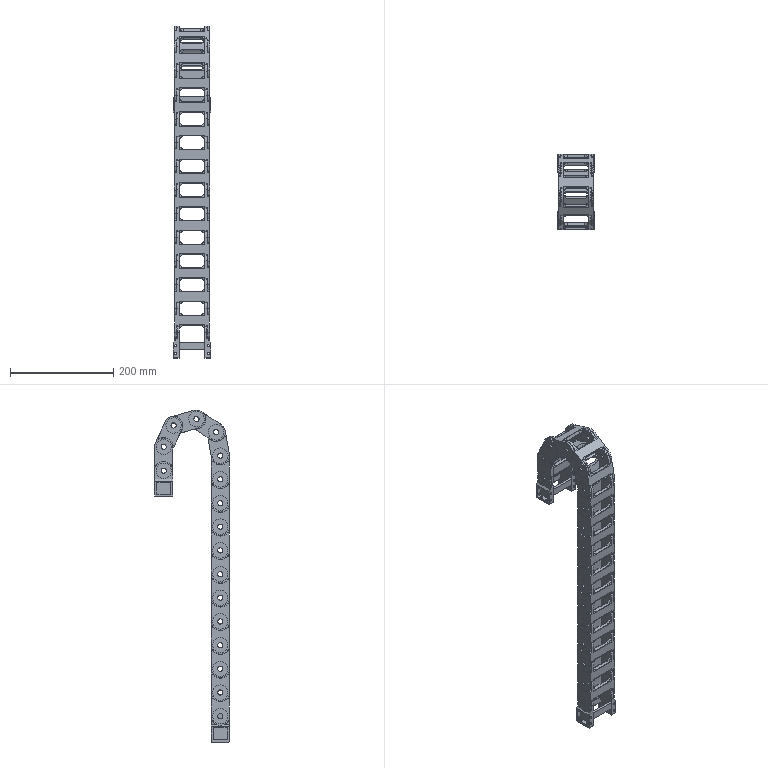Part | SolidWorks | 18 solids | 4161 faces | volume 654604 mm3 | cylinder 2259 | plane 1902 | commonest cylinder face diameters 2 x682 4.24 x192 18.2 x136 32.34 x132 10 x128 13.7 x128